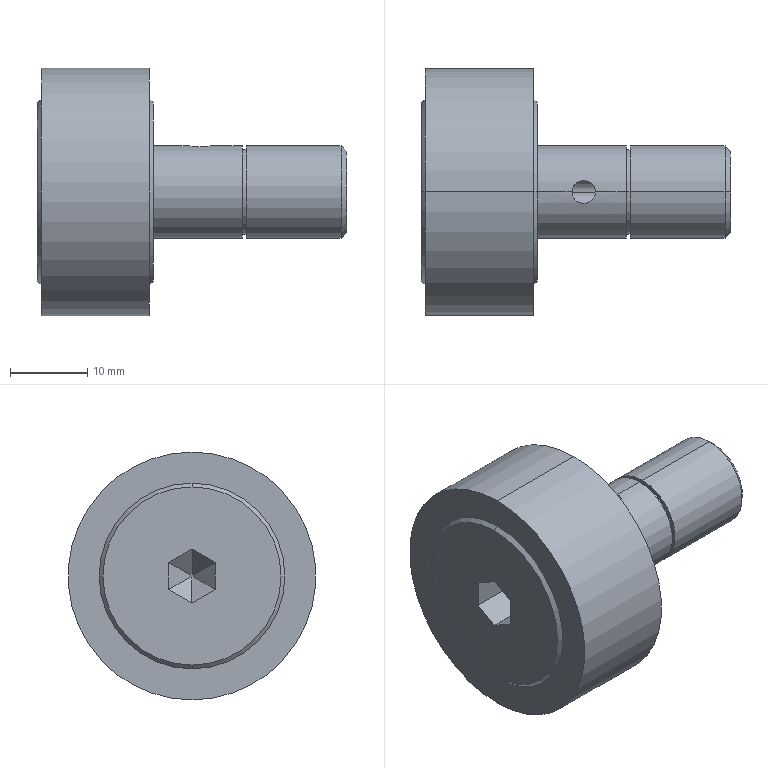Part | STEP file | BTL-01-32-0 | 1 solid | 43 faces | box 40 x 32 x 32 mm | volume 13951 mm3 | plane 21 | cylinder 14 | cone 8 | commonest cylinder face diameters 3 x4 12 x4 6 x2 11 x2 32 x2
STEP:
#1=CARTESIAN_POINT('',(7.,0.,16.));
#2=VERTEX_POINT('',#1);
#3=CARTESIAN_POINT('',(7.,0.,-16.));
#4=VERTEX_POINT('',#3);
#5=CARTESIAN_POINT('',(7.,0.,0.));
#6=DIRECTION('',(-1.,0.,0.));
#7=DIRECTION('',(0.,0.,1.));
#8=AXIS2_PLACEMENT_3D('',#5,#6,#7);
#9=CIRCLE('',#8,16.);
#10=EDGE_CURVE('',#2,#4,#9,.T.);
#11=ORIENTED_EDGE('',*,*,#10,.T.);
#12=CARTESIAN_POINT('',(-7.,0.,-16.));
#13=VERTEX_POINT('',#12);
#14=CARTESIAN_POINT('',(34.5,0.,-16.));
#15=DIRECTION('',(-1.,0.,0.));
#16=VECTOR('',#15,1000.);
#17=LINE('',#14,#16);
#18=EDGE_CURVE('',#4,#13,#17,.T.);
#19=ORIENTED_EDGE('',*,*,#18,.T.);
#20=CARTESIAN_POINT('',(-7.,0.,16.));
#21=VERTEX_POINT('',#20);
#22=CARTESIAN_POINT('',(-7.,0.,0.));
#23=DIRECTION('',(1.,0.,0.));
#24=DIRECTION('',(0.,0.,1.));
#25=AXIS2_PLACEMENT_3D('',#22,#23,#24);
#26=CIRCLE('',#25,16.);
#27=EDGE_CURVE('',#13,#21,#26,.T.);
#28=ORIENTED_EDGE('',*,*,#27,.T.);
#29=CARTESIAN_POINT('',(34.5,0.,16.));
#30=DIRECTION('',(-1.,0.,0.));
#31=VECTOR('',#30,1000.);
#32=LINE('',#29,#31);
#33=EDGE_CURVE('',#2,#21,#32,.T.);
#34=ORIENTED_EDGE('',*,*,#33,.F.);
#35=EDGE_LOOP('',(#11,#19,#28,#34));
#36=FACE_OUTER_BOUND('',#35,.T.);
#37=CARTESIAN_POINT('',(34.5,0.,0.));
#38=DIRECTION('',(-1.,0.,0.));
#39=DIRECTION('',(0.,0.,1.));
#40=AXIS2_PLACEMENT_3D('',#37,#38,#39);
#41=CYLINDRICAL_SURFACE('',#40,16.);
#42=ADVANCED_FACE('',(#36),#41,.T.);
#43=CARTESIAN_POINT('',(-7.5,0.,-11.5));
#44=VERTEX_POINT('',#43);
#45=CARTESIAN_POINT('',(-7.5,0.,11.5));
#46=VERTEX_POINT('',#45);
#47=CARTESIAN_POINT('',(-7.5,0.,0.));
#48=DIRECTION('',(1.,0.,0.));
#49=DIRECTION('',(0.,0.,-1.));
#50=AXIS2_PLACEMENT_3D('',#47,#48,#49);
#51=CIRCLE('',#50,11.5);
#52=EDGE_CURVE('',#44,#46,#51,.T.);
#53=ORIENTED_EDGE('',*,*,#52,.T.);
#54=CARTESIAN_POINT('',(-7.,0.,12.));
#55=VERTEX_POINT('',#54);
#56=CARTESIAN_POINT('',(-7.,0.,12.));
#57=DIRECTION('',(0.7071,0.,0.7071));
#58=VECTOR('',#57,1000.);
#59=LINE('',#56,#58);
#60=EDGE_CURVE('',#46,#55,#59,.T.);
#61=ORIENTED_EDGE('',*,*,#60,.T.);
#62=CARTESIAN_POINT('',(-7.,0.,-12.));
#63=VERTEX_POINT('',#62);
#64=CARTESIAN_POINT('',(-7.,0.,0.));
#65=DIRECTION('',(1.,0.,0.));
#66=DIRECTION('',(0.,0.,-1.));
#67=AXIS2_PLACEMENT_3D('',#64,#65,#66);
#68=CIRCLE('',#67,12.);
#69=EDGE_CURVE('',#63,#55,#68,.T.);
#70=ORIENTED_EDGE('',*,*,#69,.F.);
#71=CARTESIAN_POINT('',(-7.,0.,-12.));
#72=DIRECTION('',(0.7071,0.,-0.7071));
#73=VECTOR('',#72,1000.);
#74=LINE('',#71,#73);
#75=EDGE_CURVE('',#44,#63,#74,.T.);
#76=ORIENTED_EDGE('',*,*,#75,.F.);
#77=EDGE_LOOP('',(#53,#61,#70,#76));
#78=FACE_OUTER_BOUND('',#77,.T.);
#79=CARTESIAN_POINT('',(-7.,0.,0.));
#80=DIRECTION('',(1.,0.,0.));
#81=DIRECTION('',(0.,0.,-1.));
#82=AXIS2_PLACEMENT_3D('',#79,#80,#81);
#83=CONICAL_SURFACE('',#82,12.,0.7854);
#84=ADVANCED_FACE('',(#78),#83,.T.);
#85=CARTESIAN_POINT('',(7.5,0.,11.5));
#86=VERTEX_POINT('',#85);
#87=CARTESIAN_POINT('',(7.5,0.,-11.5));
#88=VERTEX_POINT('',#87);
#89=CARTESIAN_POINT('',(7.5,0.,0.));
#90=DIRECTION('',(-1.,0.,0.));
#91=DIRECTION('',(0.,0.,1.));
#92=AXIS2_PLACEMENT_3D('',#89,#90,#91);
#93=CIRCLE('',#92,11.5);
#94=EDGE_CURVE('',#86,#88,#93,.T.);
#95=ORIENTED_EDGE('',*,*,#94,.T.);
#96=CARTESIAN_POINT('',(7.,0.,-12.));
#97=VERTEX_POINT('',#96);
#98=CARTESIAN_POINT('',(7.,0.,-12.));
#99=DIRECTION('',(-0.7071,0.,-0.7071));
#100=VECTOR('',#99,1000.);
#101=LINE('',#98,#100);
#102=EDGE_CURVE('',#88,#97,#101,.T.);
#103=ORIENTED_EDGE('',*,*,#102,.T.);
#104=CARTESIAN_POINT('',(7.,0.,12.));
#105=VERTEX_POINT('',#104);
#106=CARTESIAN_POINT('',(7.,0.,0.));
#107=DIRECTION('',(1.,0.,0.));
#108=DIRECTION('',(0.,0.,1.));
#109=AXIS2_PLACEMENT_3D('',#106,#107,#108);
#110=CIRCLE('',#109,12.);
#111=EDGE_CURVE('',#97,#105,#110,.T.);
#112=ORIENTED_EDGE('',*,*,#111,.T.);
#113=CARTESIAN_POINT('',(7.,0.,12.));
#114=DIRECTION('',(-0.7071,0.,0.7071));
#115=VECTOR('',#114,1000.);
#116=LINE('',#113,#115);
#117=EDGE_CURVE('',#86,#105,#116,.T.);
#118=ORIENTED_EDGE('',*,*,#117,.F.);
#119=EDGE_LOOP('',(#95,#103,#112,#118));
#120=FACE_OUTER_BOUND('',#119,.T.);
#121=CARTESIAN_POINT('',(7.,0.,0.));
#122=DIRECTION('',(-1.,0.,0.));
#123=DIRECTION('',(0.,0.,1.));
#124=AXIS2_PLACEMENT_3D('',#121,#122,#123);
#125=CONICAL_SURFACE('',#124,12.,0.7854);
#126=ADVANCED_FACE('',(#120),#125,.T.);
#127=CARTESIAN_POINT('',(19.,0.,6.));
#128=VERTEX_POINT('',#127);
#129=CARTESIAN_POINT('',(19.,0.,-6.));
#130=VERTEX_POINT('',#129);
#131=CARTESIAN_POINT('',(19.,0.,0.));
#132=DIRECTION('',(-1.,0.,0.));
#133=DIRECTION('',(0.,0.,1.));
#134=AXIS2_PLACEMENT_3D('',#131,#132,#133);
#135=CIRCLE('',#134,6.);
#136=EDGE_CURVE('',#128,#130,#135,.T.);
#137=ORIENTED_EDGE('',*,*,#136,.T.);
#138=CARTESIAN_POINT('',(7.5,0.,-6.));
#139=VERTEX_POINT('',#138);
#140=CARTESIAN_POINT('',(34.5,0.,-6.));
#141=DIRECTION('',(-1.,0.,0.));
#142=VECTOR('',#141,1000.);
#143=LINE('',#140,#142);
#144=EDGE_CURVE('',#130,#139,#143,.T.);
#145=ORIENTED_EDGE('',*,*,#144,.T.);
#146=CARTESIAN_POINT('',(7.5,0.,6.));
#147=VERTEX_POINT('',#146);
#148=CARTESIAN_POINT('',(7.5,0.,0.));
#149=DIRECTION('',(1.,0.,0.));
#150=DIRECTION('',(0.,0.,1.));
#151=AXIS2_PLACEMENT_3D('',#148,#149,#150);
#152=CIRCLE('',#151,6.);
#153=EDGE_CURVE('',#139,#147,#152,.T.);
#154=ORIENTED_EDGE('',*,*,#153,.T.);
#155=CARTESIAN_POINT('',(12.,0.,6.));
#156=VERTEX_POINT('',#155);
#157=CARTESIAN_POINT('',(34.5,0.,6.));
#158=DIRECTION('',(-1.,0.,0.));
#159=VECTOR('',#158,1000.);
#160=LINE('',#157,#159);
#161=EDGE_CURVE('',#156,#147,#160,.T.);
#162=ORIENTED_EDGE('',*,*,#161,.F.);
#163=CARTESIAN_POINT('',(15.,0.,6.));
#164=VERTEX_POINT('',#163);
#165=CARTESIAN_POINT('',(12.,0.,6.));
#166=CARTESIAN_POINT('',(12.,0.09826,6.));
#167=CARTESIAN_POINT('',(12.01,0.1981,5.998));
#168=CARTESIAN_POINT('',(12.048,0.3907,5.988));
#169=CARTESIAN_POINT('',(12.077,0.4844,5.981));
#170=CARTESIAN_POINT('',(12.19,0.7575,5.955));
#171=CARTESIAN_POINT('',(12.301,0.9223,5.93));
#172=CARTESIAN_POINT('',(12.509,1.131,5.893));
#173=CARTESIAN_POINT('',(12.585,1.192,5.881));
#174=CARTESIAN_POINT('',(12.747,1.301,5.858));
#175=CARTESIAN_POINT('',(12.835,1.348,5.847));
#176=CARTESIAN_POINT('',(13.106,1.461,5.82));
#177=CARTESIAN_POINT('',(13.302,1.5,5.809));
#178=CARTESIAN_POINT('',(13.601,1.5,5.809));
#179=CARTESIAN_POINT('',(13.699,1.49,5.812));
#180=CARTESIAN_POINT('',(13.891,1.452,5.822));
#181=CARTESIAN_POINT('',(13.986,1.422,5.829));
#182=CARTESIAN_POINT('',(14.168,1.347,5.847));
#183=CARTESIAN_POINT('',(14.253,1.301,5.858));
#184=CARTESIAN_POINT('',(14.416,1.192,5.881));
#185=CARTESIAN_POINT('',(14.493,1.129,5.893));
#186=CARTESIAN_POINT('',(14.699,0.9219,5.93));
#187=CARTESIAN_POINT('',(14.811,0.7551,5.955));
#188=CARTESIAN_POINT('',(14.96,0.3944,5.99));
#189=CARTESIAN_POINT('',(15.,0.1965,6.));
#190=CARTESIAN_POINT('',(15.,0.,6.));
#191=B_SPLINE_CURVE_WITH_KNOTS('',3,(#165,#166,#167,#168,#169,#170,#171,#172,#173,#174,#175,#176,#177,#178,#179,#180,#181,#182,#183,#184,#185,#186,#187,#188,#189,#190),.UNSPECIFIED.,.F.,.F.,(4,2,2,2,2,2,2,2,2,2,2,2,4),(0.007062,0.007356,0.00765,0.008238,0.008533,0.008827,0.009415,0.009709,0.01,0.0103,0.01059,0.01118,0.01177),.UNSPECIFIED.);
#192=EDGE_CURVE('',#156,#164,#191,.T.);
#193=ORIENTED_EDGE('',*,*,#192,.T.);
#194=CARTESIAN_POINT('',(34.5,0.,6.));
#195=DIRECTION('',(-1.,0.,0.));
#196=VECTOR('',#195,1000.);
#197=LINE('',#194,#196);
#198=EDGE_CURVE('',#128,#164,#197,.T.);
#199=ORIENTED_EDGE('',*,*,#198,.F.);
#200=EDGE_LOOP('',(#137,#145,#154,#162,#193,#199));
#201=FACE_OUTER_BOUND('',#200,.T.);
#202=CARTESIAN_POINT('',(34.5,0.,0.));
#203=DIRECTION('',(-1.,0.,0.));
#204=DIRECTION('',(0.,0.,1.));
#205=AXIS2_PLACEMENT_3D('',#202,#203,#204);
#206=CYLINDRICAL_SURFACE('',#205,6.);
#207=ADVANCED_FACE('',(#201),#206,.T.);
#208=CARTESIAN_POINT('',(12.,0.,1.5));
#209=VERTEX_POINT('',#208);
#210=CARTESIAN_POINT('',(13.5,-1.5,0.));
#211=VERTEX_POINT('',#210);
#212=CARTESIAN_POINT('',(12.,0.,1.5));
#213=CARTESIAN_POINT('',(12.,-0.8787,1.5));
#214=CARTESIAN_POINT('',(12.621,-1.5,0.8787));
#215=CARTESIAN_POINT('',(13.5,-1.5,0.));
#216=(BOUNDED_CURVE()B_SPLINE_CURVE(3,(#212,#213,#214,#215),.UNSPECIFIED.,.F.,.F.)B_SPLINE_CURVE_WITH_KNOTS((4,4),(0.,1.571),.UNSPECIFIED.)CURVE()GEOMETRIC_REPRESENTATION_ITEM()RATIONAL_B_SPLINE_CURVE((1.,0.8047,0.8047,1.))REPRESENTATION_ITEM(''));
#217=EDGE_CURVE('',#209,#211,#216,.T.);
#218=ORIENTED_EDGE('',*,*,#217,.F.);
#219=CARTESIAN_POINT('',(12.,0.,-0.325));
#220=DIRECTION('',(0.,0.,1.));
#221=VECTOR('',#220,1000.);
#222=LINE('',#219,#221);
#223=EDGE_CURVE('',#209,#156,#222,.T.);
#224=ORIENTED_EDGE('',*,*,#223,.T.);
#225=CARTESIAN_POINT('',(15.,0.,6.));
#226=CARTESIAN_POINT('',(15.,-0.09825,6.));
#227=CARTESIAN_POINT('',(14.99,-0.1981,5.998));
#228=CARTESIAN_POINT('',(14.952,-0.3907,5.988));
#229=CARTESIAN_POINT('',(14.923,-0.4844,5.981));
#230=CARTESIAN_POINT('',(14.81,-0.7575,5.955));
#231=CARTESIAN_POINT('',(14.699,-0.9223,5.93));
#232=CARTESIAN_POINT('',(14.491,-1.131,5.893));
#233=CARTESIAN_POINT('',(14.415,-1.192,5.881));
#234=CARTESIAN_POINT('',(14.253,-1.301,5.858));
#235=CARTESIAN_POINT('',(14.165,-1.348,5.847));
#236=CARTESIAN_POINT('',(13.894,-1.461,5.82));
#237=CARTESIAN_POINT('',(13.698,-1.5,5.809));
#238=CARTESIAN_POINT('',(13.399,-1.5,5.809));
#239=CARTESIAN_POINT('',(13.301,-1.49,5.812));
#240=CARTESIAN_POINT('',(13.109,-1.452,5.822));
#241=CARTESIAN_POINT('',(13.014,-1.422,5.829));
#242=CARTESIAN_POINT('',(12.832,-1.347,5.847));
#243=CARTESIAN_POINT('',(12.747,-1.301,5.858));
#244=CARTESIAN_POINT('',(12.584,-1.192,5.881));
#245=CARTESIAN_POINT('',(12.507,-1.129,5.893));
#246=CARTESIAN_POINT('',(12.301,-0.9219,5.93));
#247=CARTESIAN_POINT('',(12.189,-0.7551,5.955));
#248=CARTESIAN_POINT('',(12.04,-0.3944,5.99));
#249=CARTESIAN_POINT('',(12.,-0.1965,6.));
#250=CARTESIAN_POINT('',(12.,0.,6.));
#251=B_SPLINE_CURVE_WITH_KNOTS('',3,(#225,#226,#227,#228,#229,#230,#231,#232,#233,#234,#235,#236,#237,#238,#239,#240,#241,#242,#243,#244,#245,#246,#247,#248,#249,#250),.UNSPECIFIED.,.F.,.F.,(4,2,2,2,2,2,2,2,2,2,2,2,4),(0.002355,0.002649,0.002943,0.003532,0.003826,0.00412,0.004708,0.005002,0.005297,0.005591,0.005885,0.006473,0.007062),.UNSPECIFIED.);
#252=EDGE_CURVE('',#164,#156,#251,.T.);
#253=ORIENTED_EDGE('',*,*,#252,.F.);
#254=CARTESIAN_POINT('',(15.,0.,1.5));
#255=VERTEX_POINT('',#254);
#256=CARTESIAN_POINT('',(15.,0.,-0.325));
#257=DIRECTION('',(0.,0.,1.));
#258=VECTOR('',#257,1000.);
#259=LINE('',#256,#258);
#260=EDGE_CURVE('',#255,#164,#259,.T.);
#261=ORIENTED_EDGE('',*,*,#260,.F.);
#262=CARTESIAN_POINT('',(13.5,-1.5,0.));
#263=CARTESIAN_POINT('',(14.379,-1.5,0.8787));
#264=CARTESIAN_POINT('',(15.,-0.8787,1.5));
#265=CARTESIAN_POINT('',(15.,0.,1.5));
#266=(BOUNDED_CURVE()B_SPLINE_CURVE(3,(#262,#263,#264,#265),.UNSPECIFIED.,.F.,.F.)B_SPLINE_CURVE_WITH_KNOTS((4,4),(1.571,3.142),.UNSPECIFIED.)CURVE()GEOMETRIC_REPRESENTATION_ITEM()RATIONAL_B_SPLINE_CURVE((1.,0.8047,0.8047,1.))REPRESENTATION_ITEM(''));
#267=EDGE_CURVE('',#211,#255,#266,.T.);
#268=ORIENTED_EDGE('',*,*,#267,.F.);
#269=EDGE_LOOP('',(#218,#224,#253,#261,#268));
#270=FACE_OUTER_BOUND('',#269,.T.);
#271=CARTESIAN_POINT('',(13.5,0.,-0.325));
#272=DIRECTION('',(0.,0.,1.));
#273=DIRECTION('',(1.,0.,0.));
#274=AXIS2_PLACEMENT_3D('',#271,#272,#273);
#275=CYLINDRICAL_SURFACE('',#274,1.5);
#276=ADVANCED_FACE('',(#270),#275,.F.);
#277=CARTESIAN_POINT('',(23.902,0.,-1.5));
#278=VERTEX_POINT('',#277);
#279=CARTESIAN_POINT('',(23.902,0.,1.5));
#280=VERTEX_POINT('',#279);
#281=CARTESIAN_POINT('',(23.902,0.,0.));
#282=DIRECTION('',(-1.,0.,0.));
#283=DIRECTION('',(0.,0.,1.));
#284=AXIS2_PLACEMENT_3D('',#281,#282,#283);
#285=CIRCLE('',#284,1.5);
#286=EDGE_CURVE('',#278,#280,#285,.T.);
#287=ORIENTED_EDGE('',*,*,#286,.F.);
#288=CARTESIAN_POINT('',(7.5,0.,-1.5));
#289=VERTEX_POINT('',#288);
#290=CARTESIAN_POINT('',(33.75,0.,-1.5));
#291=DIRECTION('',(-1.,0.,0.));
#292=VECTOR('',#291,1000.);
#293=LINE('',#290,#292);
#294=EDGE_CURVE('',#278,#289,#293,.T.);
#295=ORIENTED_EDGE('',*,*,#294,.T.);
#296=CARTESIAN_POINT('',(7.5,0.,1.5));
#297=VERTEX_POINT('',#296);
#298=CARTESIAN_POINT('',(7.5,0.,0.));
#299=DIRECTION('',(1.,0.,0.));
#300=DIRECTION('',(0.,0.,1.));
#301=AXIS2_PLACEMENT_3D('',#298,#299,#300);
#302=CIRCLE('',#301,1.5);
#303=EDGE_CURVE('',#297,#289,#302,.T.);
#304=ORIENTED_EDGE('',*,*,#303,.F.);
#305=CARTESIAN_POINT('',(33.75,0.,1.5));
#306=DIRECTION('',(-1.,0.,0.));
#307=VECTOR('',#306,1000.);
#308=LINE('',#305,#307);
#309=EDGE_CURVE('',#209,#297,#308,.T.);
#310=ORIENTED_EDGE('',*,*,#309,.F.);
#311=ORIENTED_EDGE('',*,*,#217,.T.);
#312=ORIENTED_EDGE('',*,*,#267,.T.);
#313=CARTESIAN_POINT('',(33.75,0.,1.5));
#314=DIRECTION('',(-1.,0.,0.));
#315=VECTOR('',#314,1000.);
#316=LINE('',#313,#315);
#317=EDGE_CURVE('',#280,#255,#316,.T.);
#318=ORIENTED_EDGE('',*,*,#317,.F.);
#319=EDGE_LOOP('',(#287,#295,#304,#310,#311,#312,#318));
#320=FACE_OUTER_BOUND('',#319,.T.);
#321=CARTESIAN_POINT('',(33.75,0.,0.));
#322=DIRECTION('',(-1.,0.,0.));
#323=DIRECTION('',(0.,0.,1.));
#324=AXIS2_PLACEMENT_3D('',#321,#322,#323);
#325=CYLINDRICAL_SURFACE('',#324,1.5);
#326=ADVANCED_FACE('',(#320),#325,.F.);
#327=CARTESIAN_POINT('',(19.5,0.,5.5));
#328=VERTEX_POINT('',#327);
#329=CARTESIAN_POINT('',(19.5,0.,-5.5));
#330=VERTEX_POINT('',#329);
#331=CARTESIAN_POINT('',(19.5,0.,0.));
#332=DIRECTION('',(-1.,0.,0.));
#333=DIRECTION('',(0.,0.,1.));
#334=AXIS2_PLACEMENT_3D('',#331,#332,#333);
#335=CIRCLE('',#334,5.5);
#336=EDGE_CURVE('',#328,#330,#335,.T.);
#337=ORIENTED_EDGE('',*,*,#336,.T.);
#338=CARTESIAN_POINT('',(19.,0.,-5.5));
#339=VERTEX_POINT('',#338);
#340=CARTESIAN_POINT('',(34.5,0.,-5.5));
#341=DIRECTION('',(-1.,0.,0.));
#342=VECTOR('',#341,1000.);
#343=LINE('',#340,#342);
#344=EDGE_CURVE('',#330,#339,#343,.T.);
#345=ORIENTED_EDGE('',*,*,#344,.T.);
#346=CARTESIAN_POINT('',(19.,0.,5.5));
#347=VERTEX_POINT('',#346);
#348=CARTESIAN_POINT('',(19.,0.,0.));
#349=DIRECTION('',(1.,0.,0.));
#350=DIRECTION('',(0.,0.,1.));
#351=AXIS2_PLACEMENT_3D('',#348,#349,#350);
#352=CIRCLE('',#351,5.5);
#353=EDGE_CURVE('',#339,#347,#352,.T.);
#354=ORIENTED_EDGE('',*,*,#353,.T.);
#355=CARTESIAN_POINT('',(34.5,0.,5.5));
#356=DIRECTION('',(-1.,0.,0.));
#357=VECTOR('',#356,1000.);
#358=LINE('',#355,#357);
#359=EDGE_CURVE('',#328,#347,#358,.T.);
#360=ORIENTED_EDGE('',*,*,#359,.F.);
#361=EDGE_LOOP('',(#337,#345,#354,#360));
#362=FACE_OUTER_BOUND('',#361,.T.);
#363=CARTESIAN_POINT('',(34.5,0.,0.));
#364=DIRECTION('',(-1.,0.,0.));
#365=DIRECTION('',(0.,0.,1.));
#366=AXIS2_PLACEMENT_3D('',#363,#364,#365);
#367=CYLINDRICAL_SURFACE('',#366,5.5);
#368=ADVANCED_FACE('',(#362),#367,.T.);
#369=ORIENTED_EDGE('',*,*,#286,.T.);
#370=CARTESIAN_POINT('',(26.5,0.,3.));
#371=VERTEX_POINT('',#370);
#372=CARTESIAN_POINT('',(26.5,0.,3.));
#373=DIRECTION('',(0.866,0.,0.5));
#374=VECTOR('',#373,1000.);
#375=LINE('',#372,#374);
#376=EDGE_CURVE('',#280,#371,#375,.T.);
#377=ORIENTED_EDGE('',*,*,#376,.T.);
#378=CARTESIAN_POINT('',(26.5,0.,-3.));
#379=VERTEX_POINT('',#378);
#380=CARTESIAN_POINT('',(26.5,0.,0.));
#381=DIRECTION('',(-1.,0.,0.));
#382=DIRECTION('',(0.,0.,1.));
#383=AXIS2_PLACEMENT_3D('',#380,#381,#382);
#384=CIRCLE('',#383,3.);
#385=EDGE_CURVE('',#379,#371,#384,.T.);
#386=ORIENTED_EDGE('',*,*,#385,.F.);
#387=CARTESIAN_POINT('',(26.5,0.,-3.));
#388=DIRECTION('',(0.866,0.,-0.5));
#389=VECTOR('',#388,1000.);
#390=LINE('',#387,#389);
#391=EDGE_CURVE('',#278,#379,#390,.T.);
#392=ORIENTED_EDGE('',*,*,#391,.F.);
#393=EDGE_LOOP('',(#369,#377,#386,#392));
#394=FACE_OUTER_BOUND('',#393,.T.);
#395=CARTESIAN_POINT('',(26.5,0.,0.));
#396=DIRECTION('',(1.,0.,0.));
#397=DIRECTION('',(0.,0.,-1.));
#398=AXIS2_PLACEMENT_3D('',#395,#396,#397);
#399=CONICAL_SURFACE('',#398,3.,0.5236);
#400=ADVANCED_FACE('',(#394),#399,.F.);
#401=CARTESIAN_POINT('',(32.5,0.,-3.));
#402=VERTEX_POINT('',#401);
#403=CARTESIAN_POINT('',(32.5,0.,3.));
#404=VERTEX_POINT('',#403);
#405=CARTESIAN_POINT('',(32.5,0.,0.));
#406=DIRECTION('',(-1.,0.,0.));
#407=DIRECTION('',(0.,0.,1.));
#408=AXIS2_PLACEMENT_3D('',#405,#406,#407);
#409=CIRCLE('',#408,3.);
#410=EDGE_CURVE('',#402,#404,#409,.T.);
#411=ORIENTED_EDGE('',*,*,#410,.F.);
#412=CARTESIAN_POINT('',(33.75,0.,-3.));
#413=DIRECTION('',(-1.,0.,0.));
#414=VECTOR('',#413,1000.);
#415=LINE('',#412,#414);
#416=EDGE_CURVE('',#402,#379,#415,.T.);
#417=ORIENTED_EDGE('',*,*,#416,.T.);
#418=ORIENTED_EDGE('',*,*,#385,.T.);
#419=CARTESIAN_POINT('',(33.75,0.,3.));
#420=DIRECTION('',(-1.,0.,0.));
#421=VECTOR('',#420,1000.);
#422=LINE('',#419,#421);
#423=EDGE_CURVE('',#404,#371,#422,.T.);
#424=ORIENTED_EDGE('',*,*,#423,.F.);
#425=EDGE_LOOP('',(#411,#417,#418,#424));
#426=FACE_OUTER_BOUND('',#425,.T.);
#427=CARTESIAN_POINT('',(33.75,0.,0.));
#428=DIRECTION('',(-1.,0.,0.));
#429=DIRECTION('',(0.,0.,1.));
#430=AXIS2_PLACEMENT_3D('',#427,#428,#429);
#431=CYLINDRICAL_SURFACE('',#430,3.);
#432=ADVANCED_FACE('',(#426),#431,.F.);
#433=CARTESIAN_POINT('',(31.75,0.,6.));
#434=VERTEX_POINT('',#433);
#435=CARTESIAN_POINT('',(31.75,0.,-6.));
#436=VERTEX_POINT('',#435);
#437=CARTESIAN_POINT('',(31.75,0.,0.));
#438=DIRECTION('',(-1.,0.,0.));
#439=DIRECTION('',(0.,0.,1.));
#440=AXIS2_PLACEMENT_3D('',#437,#438,#439);
#441=CIRCLE('',#440,6.);
#442=EDGE_CURVE('',#434,#436,#441,.T.);
#443=ORIENTED_EDGE('',*,*,#442,.T.);
#444=CARTESIAN_POINT('',(19.5,0.,-6.));
#445=VERTEX_POINT('',#444);
#446=CARTESIAN_POINT('',(34.5,0.,-6.));
#447=DIRECTION('',(-1.,0.,0.));
#448=VECTOR('',#447,1000.);
#449=LINE('',#446,#448);
#450=EDGE_CURVE('',#436,#445,#449,.T.);
#451=ORIENTED_EDGE('',*,*,#450,.T.);
#452=CARTESIAN_POINT('',(19.5,0.,6.));
#453=VERTEX_POINT('',#452);
#454=CARTESIAN_POINT('',(19.5,0.,0.));
#455=DIRECTION('',(-1.,0.,0.));
#456=DIRECTION('',(0.,0.,1.));
#457=AXIS2_PLACEMENT_3D('',#454,#455,#456);
#458=CIRCLE('',#457,6.);
#459=EDGE_CURVE('',#453,#445,#458,.T.);
#460=ORIENTED_EDGE('',*,*,#459,.F.);
#461=CARTESIAN_POINT('',(34.5,0.,6.));
#462=DIRECTION('',(-1.,0.,0.));
#463=VECTOR('',#462,1000.);
#464=LINE('',#461,#463);
#465=EDGE_CURVE('',#434,#453,#464,.T.);
#466=ORIENTED_EDGE('',*,*,#465,.F.);
#467=EDGE_LOOP('',(#443,#451,#460,#466));
#468=FACE_OUTER_BOUND('',#467,.T.);
#469=CARTESIAN_POINT('',(34.5,0.,0.));
#470=DIRECTION('',(-1.,0.,0.));
#471=DIRECTION('',(0.,0.,1.));
#472=AXIS2_PLACEMENT_3D('',#469,#470,#471);
#473=CYLINDRICAL_SURFACE('',#472,6.);
#474=ADVANCED_FACE('',(#468),#473,.T.);
#475=CARTESIAN_POINT('',(32.5,0.,5.25));
#476=VERTEX_POINT('',#475);
#477=CARTESIAN_POINT('',(32.5,0.,-5.25));
#478=VERTEX_POINT('',#477);
#479=CARTESIAN_POINT('',(32.5,0.,0.));
#480=DIRECTION('',(-1.,0.,0.));
#481=DIRECTION('',(0.,0.,1.));
#482=AXIS2_PLACEMENT_3D('',#479,#480,#481);
#483=CIRCLE('',#482,5.25);
#484=EDGE_CURVE('',#476,#478,#483,.T.);
#485=ORIENTED_EDGE('',*,*,#484,.T.);
#486=CARTESIAN_POINT('',(31.75,0.,-6.));
#487=DIRECTION('',(-0.7071,0.,-0.7071));
#488=VECTOR('',#487,1000.);
#489=LINE('',#486,#488);
#490=EDGE_CURVE('',#478,#436,#489,.T.);
#491=ORIENTED_EDGE('',*,*,#490,.T.);
#492=ORIENTED_EDGE('',*,*,#442,.F.);
#493=CARTESIAN_POINT('',(31.75,0.,6.));
#494=DIRECTION('',(-0.7071,0.,0.7071));
#495=VECTOR('',#494,1000.);
#496=LINE('',#493,#495);
#497=EDGE_CURVE('',#476,#434,#496,.T.);
#498=ORIENTED_EDGE('',*,*,#497,.F.);
#499=EDGE_LOOP('',(#485,#491,#492,#498));
#500=FACE_OUTER_BOUND('',#499,.T.);
#501=CARTESIAN_POINT('',(31.75,0.,0.));
#502=DIRECTION('',(-1.,0.,0.));
#503=DIRECTION('',(0.,0.,1.));
#504=AXIS2_PLACEMENT_3D('',#501,#502,#503);
#505=CONICAL_SURFACE('',#504,6.,0.7854);
#506=ADVANCED_FACE('',(#500),#505,.T.);
#507=ORIENTED_EDGE('',*,*,#18,.F.);
#508=CARTESIAN_POINT('',(7.,0.,0.));
#509=DIRECTION('',(-1.,0.,0.));
#510=DIRECTION('',(0.,0.,1.));
#511=AXIS2_PLACEMENT_3D('',#508,#509,#510);
#512=CIRCLE('',#511,16.);
#513=EDGE_CURVE('',#4,#2,#512,.T.);
#514=ORIENTED_EDGE('',*,*,#513,.T.);
#515=ORIENTED_EDGE('',*,*,#33,.T.);
#516=CARTESIAN_POINT('',(-7.,0.,0.));
#517=DIRECTION('',(1.,0.,0.));
#518=DIRECTION('',(0.,0.,1.));
#519=AXIS2_PLACEMENT_3D('',#516,#517,#518);
#520=CIRCLE('',#519,16.);
#521=EDGE_CURVE('',#21,#13,#520,.T.);
#522=ORIENTED_EDGE('',*,*,#521,.T.);
#523=EDGE_LOOP('',(#507,#514,#515,#522));
#524=FACE_OUTER_BOUND('',#523,.T.);
#525=CARTESIAN_POINT('',(34.5,0.,0.));
#526=DIRECTION('',(-1.,0.,0.));
#527=DIRECTION('',(0.,0.,1.));
#528=AXIS2_PLACEMENT_3D('',#525,#526,#527);
#529=CYLINDRICAL_SURFACE('',#528,16.);
#530=ADVANCED_FACE('',(#524),#529,.T.);
#531=ORIENTED_EDGE('',*,*,#69,.T.);
#532=CARTESIAN_POINT('',(-7.,0.,0.));
#533=DIRECTION('',(1.,0.,0.));
#534=DIRECTION('',(0.,0.,-1.));
#535=AXIS2_PLACEMENT_3D('',#532,#533,#534);
#536=CIRCLE('',#535,12.);
#537=EDGE_CURVE('',#55,#63,#536,.T.);
#538=ORIENTED_EDGE('',*,*,#537,.T.);
#539=EDGE_LOOP('',(#531,#538));
#540=FACE_BOUND('',#539,.T.);
#541=ORIENTED_EDGE('',*,*,#521,.F.);
#542=ORIENTED_EDGE('',*,*,#27,.F.);
#543=EDGE_LOOP('',(#541,#542));
#544=FACE_OUTER_BOUND('',#543,.T.);
#545=CARTESIAN_POINT('',(-7.,0.,0.));
#546=DIRECTION('',(-1.,0.,0.));
#547=DIRECTION('',(0.,0.,1.));
#548=AXIS2_PLACEMENT_3D('',#545,#546,#547);
#549=PLANE('',#548);
#550=ADVANCED_FACE('',(#540,#544),#549,.T.);
#551=CARTESIAN_POINT('',(7.,0.,0.));
#552=DIRECTION('',(1.,0.,0.));
#553=DIRECTION('',(0.,0.,1.));
#554=AXIS2_PLACEMENT_3D('',#551,#552,#553);
#555=CIRCLE('',#554,12.);
#556=EDGE_CURVE('',#105,#97,#555,.T.);
#557=ORIENTED_EDGE('',*,*,#556,.F.);
#558=ORIENTED_EDGE('',*,*,#111,.F.);
#559=EDGE_LOOP('',(#557,#558));
#560=FACE_BOUND('',#559,.T.);
#561=ORIENTED_EDGE('',*,*,#10,.F.);
#562=ORIENTED_EDGE('',*,*,#513,.F.);
#563=EDGE_LOOP('',(#561,#562));
#564=FACE_OUTER_BOUND('',#563,.T.);
#565=CARTESIAN_POINT('',(7.,0.,0.));
#566=DIRECTION('',(-1.,0.,0.));
#567=DIRECTION('',(0.,0.,1.));
#568=AXIS2_PLACEMENT_3D('',#565,#566,#567);
#569=PLANE('',#568);
#570=ADVANCED_FACE('',(#560,#564),#569,.F.);
#571=ORIENTED_EDGE('',*,*,#60,.F.);
#572=CARTESIAN_POINT('',(-7.5,0.,0.));
#573=DIRECTION('',(1.,0.,0.));
#574=DIRECTION('',(0.,0.,-1.));
#575=AXIS2_PLACEMENT_3D('',#572,#573,#574);
#576=CIRCLE('',#575,11.5);
#577=EDGE_CURVE('',#46,#44,#576,.T.);
#578=ORIENTED_EDGE('',*,*,#577,.T.);
#579=ORIENTED_EDGE('',*,*,#75,.T.);
#580=ORIENTED_EDGE('',*,*,#537,.F.);
#581=EDGE_LOOP('',(#571,#578,#579,#580));
#582=FACE_OUTER_BOUND('',#581,.T.);
#583=CARTESIAN_POINT('',(-7.,0.,0.));
#584=DIRECTION('',(1.,0.,0.));
#585=DIRECTION('',(0.,0.,-1.));
#586=AXIS2_PLACEMENT_3D('',#583,#584,#585);
#587=CONICAL_SURFACE('',#586,12.,0.7854);
#588=ADVANCED_FACE('',(#582),#587,.T.);
#589=ORIENTED_EDGE('',*,*,#102,.F.);
#590=CARTESIAN_POINT('',(7.5,0.,0.));
#591=DIRECTION('',(-1.,0.,0.));
#592=DIRECTION('',(0.,0.,1.));
#593=AXIS2_PLACEMENT_3D('',#590,#591,#592);
#594=CIRCLE('',#593,11.5);
#595=EDGE_CURVE('',#88,#86,#594,.T.);
#596=ORIENTED_EDGE('',*,*,#595,.T.);
#597=ORIENTED_EDGE('',*,*,#117,.T.);
#598=ORIENTED_EDGE('',*,*,#556,.T.);
#599=EDGE_LOOP('',(#589,#596,#597,#598));
#600=FACE_OUTER_BOUND('',#599,.T.);
#601=CARTESIAN_POINT('',(7.,0.,0.));
#602=DIRECTION('',(-1.,0.,0.));
#603=DIRECTION('',(0.,0.,1.));
#604=AXIS2_PLACEMENT_3D('',#601,#602,#603);
#605=CONICAL_SURFACE('',#604,12.,0.7854);
#606=ADVANCED_FACE('',(#600),#605,.T.);
#607=CARTESIAN_POINT('',(-7.5,-3.,1.732));
#608=VERTEX_POINT('',#607);
#609=CARTESIAN_POINT('',(-7.5,-3.,-1.732));
#610=VERTEX_POINT('',#609);
#611=CARTESIAN_POINT('',(-7.5,-3.,0.));
#612=DIRECTION('',(0.,0.,-1.));
#613=VECTOR('',#612,1000.);
#614=LINE('',#611,#613);
#615=EDGE_CURVE('',#608,#610,#614,.T.);
#616=ORIENTED_EDGE('',*,*,#615,.T.);
#617=CARTESIAN_POINT('',(-7.5,0.,-3.464));
#618=VERTEX_POINT('',#617);
#619=CARTESIAN_POINT('',(-7.5,-3.,-1.732));
#620=DIRECTION('',(0.,0.866,-0.5));
#621=VECTOR('',#620,1000.);
#622=LINE('',#619,#621);
#623=EDGE_CURVE('',#610,#618,#622,.T.);
#624=ORIENTED_EDGE('',*,*,#623,.T.);
#625=CARTESIAN_POINT('',(-7.5,3.,-1.732));
#626=VERTEX_POINT('',#625);
#627=CARTESIAN_POINT('',(-7.5,0.,-3.464));
#628=DIRECTION('',(0.,0.866,0.5));
#629=VECTOR('',#628,1000.);
#630=LINE('',#627,#629);
#631=EDGE_CURVE('',#618,#626,#630,.T.);
#632=ORIENTED_EDGE('',*,*,#631,.T.);
#633=CARTESIAN_POINT('',(-7.5,3.,1.732));
#634=VERTEX_POINT('',#633);
#635=CARTESIAN_POINT('',(-7.5,3.,0.));
#636=DIRECTION('',(0.,0.,1.));
#637=VECTOR('',#636,1000.);
#638=LINE('',#635,#637);
#639=EDGE_CURVE('',#626,#634,#638,.T.);
#640=ORIENTED_EDGE('',*,*,#639,.T.);
#641=CARTESIAN_POINT('',(-7.5,0.,3.464));
#642=VERTEX_POINT('',#641);
#643=CARTESIAN_POINT('',(-7.5,3.,1.732));
#644=DIRECTION('',(0.,-0.866,0.5));
#645=VECTOR('',#644,1000.);
#646=LINE('',#643,#645);
#647=EDGE_CURVE('',#634,#642,#646,.T.);
#648=ORIENTED_EDGE('',*,*,#647,.T.);
#649=CARTESIAN_POINT('',(-7.5,0.,3.464));
#650=DIRECTION('',(0.,-0.866,-0.5));
#651=VECTOR('',#650,1000.);
#652=LINE('',#649,#651);
#653=EDGE_CURVE('',#642,#608,#652,.T.);
#654=ORIENTED_EDGE('',*,*,#653,.T.);
#655=EDGE_LOOP('',(#616,#624,#632,#640,#648,#654));
#656=FACE_BOUND('',#655,.T.);
#657=ORIENTED_EDGE('',*,*,#52,.F.);
#658=ORIENTED_EDGE('',*,*,#577,.F.);
#659=EDGE_LOOP('',(#657,#658));
#660=FACE_OUTER_BOUND('',#659,.T.);
#661=CARTESIAN_POINT('',(-7.5,0.,0.));
#662=DIRECTION('',(-1.,0.,0.));
#663=DIRECTION('',(0.,0.,1.));
#664=AXIS2_PLACEMENT_3D('',#661,#662,#663);
#665=PLANE('',#664);
#666=ADVANCED_FACE('',(#656,#660),#665,.T.);
#667=CARTESIAN_POINT('',(7.5,0.,0.));
#668=DIRECTION('',(1.,0.,0.));
#669=DIRECTION('',(0.,0.,1.));
#670=AXIS2_PLACEMENT_3D('',#667,#668,#669);
#671=CIRCLE('',#670,6.);
#672=EDGE_CURVE('',#147,#139,#671,.T.);
#673=ORIENTED_EDGE('',*,*,#672,.F.);
#674=ORIENTED_EDGE('',*,*,#153,.F.);
#675=EDGE_LOOP('',(#673,#674));
#676=FACE_BOUND('',#675,.T.);
#677=ORIENTED_EDGE('',*,*,#94,.F.);
#678=ORIENTED_EDGE('',*,*,#595,.F.);
#679=EDGE_LOOP('',(#677,#678));
#680=FACE_OUTER_BOUND('',#679,.T.);
#681=CARTESIAN_POINT('',(7.5,0.,0.));
#682=DIRECTION('',(-1.,0.,0.));
#683=DIRECTION('',(0.,0.,1.));
#684=AXIS2_PLACEMENT_3D('',#681,#682,#683);
#685=PLANE('',#684);
#686=ADVANCED_FACE('',(#676,#680),#685,.F.);
#687=ORIENTED_EDGE('',*,*,#623,.F.);
#688=CARTESIAN_POINT('',(-2.5,-3.,-1.732));
#689=VERTEX_POINT('',#688);
#690=CARTESIAN_POINT('',(-7.5,-3.,-1.732));
#691=DIRECTION('',(-1.,0.,0.));
#692=VECTOR('',#691,1000.);
#693=LINE('',#690,#692);
#694=EDGE_CURVE('',#689,#610,#693,.T.);
#695=ORIENTED_EDGE('',*,*,#694,.F.);
#696=CARTESIAN_POINT('',(-2.5,0.,-3.464));
#697=VERTEX_POINT('',#696);
#698=CARTESIAN_POINT('',(-2.5,0.,-3.464));
#699=DIRECTION('',(0.,-0.866,0.5));
#700=VECTOR('',#699,1000.);
#701=LINE('',#698,#700);
#702=EDGE_CURVE('',#697,#689,#701,.T.);
#703=ORIENTED_EDGE('',*,*,#702,.F.);
#704=CARTESIAN_POINT('',(-7.5,0.,-3.464));
#705=DIRECTION('',(1.,0.,0.));
#706=VECTOR('',#705,1000.);
#707=LINE('',#704,#706);
#708=EDGE_CURVE('',#618,#697,#707,.T.);
#709=ORIENTED_EDGE('',*,*,#708,.F.);
#710=EDGE_LOOP('',(#687,#695,#703,#709));
#711=FACE_OUTER_BOUND('',#710,.T.);
#712=CARTESIAN_POINT('',(-7.5,0.,-3.464));
#713=DIRECTION('',(0.,-0.5,-0.866));
#714=DIRECTION('',(0.,0.866,-0.5));
#715=AXIS2_PLACEMENT_3D('',#712,#713,#714);
#716=PLANE('',#715);
#717=ADVANCED_FACE('',(#711),#716,.F.);
#718=ORIENTED_EDGE('',*,*,#615,.F.);
#719=CARTESIAN_POINT('',(-2.5,-3.,1.732));
#720=VERTEX_POINT('',#719);
#721=CARTESIAN_POINT('',(-7.5,-3.,1.732));
#722=DIRECTION('',(-1.,0.,0.));
#723=VECTOR('',#722,1000.);
#724=LINE('',#721,#723);
#725=EDGE_CURVE('',#720,#608,#724,.T.);
#726=ORIENTED_EDGE('',*,*,#725,.F.);
#727=CARTESIAN_POINT('',(-2.5,-3.,-1.732));
#728=DIRECTION('',(0.,0.,1.));
#729=VECTOR('',#728,1000.);
#730=LINE('',#727,#729);
#731=EDGE_CURVE('',#689,#720,#730,.T.);
#732=ORIENTED_EDGE('',*,*,#731,.F.);
#733=ORIENTED_EDGE('',*,*,#694,.T.);
#734=EDGE_LOOP('',(#718,#726,#732,#733));
#735=FACE_OUTER_BOUND('',#734,.T.);
#736=CARTESIAN_POINT('',(-7.5,-3.,-1.732));
#737=DIRECTION('',(0.,-1.,0.));
#738=DIRECTION('',(0.,0.,-1.));
#739=AXIS2_PLACEMENT_3D('',#736,#737,#738);
#740=PLANE('',#739);
#741=ADVANCED_FACE('',(#735),#740,.F.);
#742=ORIENTED_EDGE('',*,*,#653,.F.);
#743=CARTESIAN_POINT('',(-2.5,0.,3.464));
#744=VERTEX_POINT('',#743);
#745=CARTESIAN_POINT('',(-7.5,0.,3.464));
#746=DIRECTION('',(-1.,0.,0.));
#747=VECTOR('',#746,1000.);
#748=LINE('',#745,#747);
#749=EDGE_CURVE('',#744,#642,#748,.T.);
#750=ORIENTED_EDGE('',*,*,#749,.F.);
#751=CARTESIAN_POINT('',(-2.5,-3.,1.732));
#752=DIRECTION('',(0.,0.866,0.5));
#753=VECTOR('',#752,1000.);
#754=LINE('',#751,#753);
#755=EDGE_CURVE('',#720,#744,#754,.T.);
#756=ORIENTED_EDGE('',*,*,#755,.F.);
#757=ORIENTED_EDGE('',*,*,#725,.T.);
#758=EDGE_LOOP('',(#742,#750,#756,#757));
#759=FACE_OUTER_BOUND('',#758,.T.);
#760=CARTESIAN_POINT('',(-7.5,-3.,1.732));
#761=DIRECTION('',(0.,-0.5,0.866));
#762=DIRECTION('',(0.,-0.866,-0.5));
#763=AXIS2_PLACEMENT_3D('',#760,#761,#762);
#764=PLANE('',#763);
#765=ADVANCED_FACE('',(#759),#764,.F.);
#766=ORIENTED_EDGE('',*,*,#647,.F.);
#767=CARTESIAN_POINT('',(-2.5,3.,1.732));
#768=VERTEX_POINT('',#767);
#769=CARTESIAN_POINT('',(-7.5,3.,1.732));
#770=DIRECTION('',(-1.,0.,0.));
#771=VECTOR('',#770,1000.);
#772=LINE('',#769,#771);
#773=EDGE_CURVE('',#768,#634,#772,.T.);
#774=ORIENTED_EDGE('',*,*,#773,.F.);
#775=CARTESIAN_POINT('',(-2.5,0.,3.464));
#776=DIRECTION('',(0.,0.866,-0.5));
#777=VECTOR('',#776,1000.);
#778=LINE('',#775,#777);
#779=EDGE_CURVE('',#744,#768,#778,.T.);
#780=ORIENTED_EDGE('',*,*,#779,.F.);
#781=ORIENTED_EDGE('',*,*,#749,.T.);
#782=EDGE_LOOP('',(#766,#774,#780,#781));
#783=FACE_OUTER_BOUND('',#782,.T.);
#784=CARTESIAN_POINT('',(-7.5,0.,3.464));
#785=DIRECTION('',(0.,0.5,0.866));
#786=DIRECTION('',(0.,-0.866,0.5));
#787=AXIS2_PLACEMENT_3D('',#784,#785,#786);
#788=PLANE('',#787);
#789=ADVANCED_FACE('',(#783),#788,.F.);
#790=ORIENTED_EDGE('',*,*,#639,.F.);
#791=CARTESIAN_POINT('',(-2.5,3.,-1.732));
#792=VERTEX_POINT('',#791);
#793=CARTESIAN_POINT('',(-7.5,3.,-1.732));
#794=DIRECTION('',(-1.,0.,0.));
#795=VECTOR('',#794,1000.);
#796=LINE('',#793,#795);
#797=EDGE_CURVE('',#792,#626,#796,.T.);
#798=ORIENTED_EDGE('',*,*,#797,.F.);
#799=CARTESIAN_POINT('',(-2.5,3.,1.732));
#800=DIRECTION('',(0.,0.,-1.));
#801=VECTOR('',#800,1000.);
#802=LINE('',#799,#801);
#803=EDGE_CURVE('',#768,#792,#802,.T.);
#804=ORIENTED_EDGE('',*,*,#803,.F.);
#805=ORIENTED_EDGE('',*,*,#773,.T.);
#806=EDGE_LOOP('',(#790,#798,#804,#805));
#807=FACE_OUTER_BOUND('',#806,.T.);
#808=CARTESIAN_POINT('',(-7.5,3.,1.732));
#809=DIRECTION('',(0.,1.,0.));
#810=DIRECTION('',(0.,0.,1.));
#811=AXIS2_PLACEMENT_3D('',#808,#809,#810);
#812=PLANE('',#811);
#813=ADVANCED_FACE('',(#807),#812,.F.);
#814=ORIENTED_EDGE('',*,*,#631,.F.);
#815=ORIENTED_EDGE('',*,*,#708,.T.);
#816=CARTESIAN_POINT('',(-2.5,3.,-1.732));
#817=DIRECTION('',(0.,-0.866,-0.5));
#818=VECTOR('',#817,1000.);
#819=LINE('',#816,#818);
#820=EDGE_CURVE('',#792,#697,#819,.T.);
#821=ORIENTED_EDGE('',*,*,#820,.F.);
#822=ORIENTED_EDGE('',*,*,#797,.T.);
#823=EDGE_LOOP('',(#814,#815,#821,#822));
#824=FACE_OUTER_BOUND('',#823,.T.);
#825=CARTESIAN_POINT('',(-7.5,3.,-1.732));
#826=DIRECTION('',(0.,0.5,-0.866));
#827=DIRECTION('',(0.,0.866,0.5));
#828=AXIS2_PLACEMENT_3D('',#825,#826,#827);
#829=PLANE('',#828);
#830=ADVANCED_FACE('',(#824),#829,.F.);
#831=ORIENTED_EDGE('',*,*,#144,.F.);
#832=CARTESIAN_POINT('',(19.,0.,0.));
#833=DIRECTION('',(-1.,0.,0.));
#834=DIRECTION('',(0.,0.,1.));
#835=AXIS2_PLACEMENT_3D('',#832,#833,#834);
#836=CIRCLE('',#835,6.);
#837=EDGE_CURVE('',#130,#128,#836,.T.);
#838=ORIENTED_EDGE('',*,*,#837,.T.);
#839=ORIENTED_EDGE('',*,*,#198,.T.);
#840=ORIENTED_EDGE('',*,*,#252,.T.);
#841=ORIENTED_EDGE('',*,*,#161,.T.);
#842=ORIENTED_EDGE('',*,*,#672,.T.);
#843=EDGE_LOOP('',(#831,#838,#839,#840,#841,#842));
#844=FACE_OUTER_BOUND('',#843,.T.);
#845=CARTESIAN_POINT('',(34.5,0.,0.));
#846=DIRECTION('',(-1.,0.,0.));
#847=DIRECTION('',(0.,0.,1.));
#848=AXIS2_PLACEMENT_3D('',#845,#846,#847);
#849=CYLINDRICAL_SURFACE('',#848,6.);
#850=ADVANCED_FACE('',(#844),#849,.T.);
#851=CARTESIAN_POINT('',(0.5,0.,-0.25));
#852=VERTEX_POINT('',#851);
#853=CARTESIAN_POINT('',(0.5,-0.2165,-0.125));
#854=VERTEX_POINT('',#853);
#855=CARTESIAN_POINT('',(0.5,0.,-0.25));
#856=DIRECTION('',(0.,-0.866,0.5));
#857=VECTOR('',#856,1000.);
#858=LINE('',#855,#857);
#859=EDGE_CURVE('',#852,#854,#858,.T.);
#860=ORIENTED_EDGE('',*,*,#859,.F.);
#861=CARTESIAN_POINT('',(-0.7684,0.,-1.609));
#862=DIRECTION('',(0.6823,0.,0.731));
#863=VECTOR('',#862,1000.);
#864=LINE('',#861,#863);
#865=EDGE_CURVE('',#697,#852,#864,.T.);
#866=ORIENTED_EDGE('',*,*,#865,.F.);
#867=ORIENTED_EDGE('',*,*,#702,.T.);
#868=CARTESIAN_POINT('',(0.5,-0.2165,-0.125));
#869=DIRECTION('',(-0.6823,-0.6331,-0.3655));
#870=VECTOR('',#869,1000.);
#871=LINE('',#868,#870);
#872=EDGE_CURVE('',#854,#689,#871,.T.);
#873=ORIENTED_EDGE('',*,*,#872,.F.);
#874=EDGE_LOOP('',(#860,#866,#867,#873));
#875=FACE_OUTER_BOUND('',#874,.T.);
#876=CARTESIAN_POINT('',(-1.,-0.8041,-1.393));
#877=DIRECTION('',(0.6802,-0.3665,-0.6349));
#878=DIRECTION('',(-0.6823,0.,-0.731));
#879=AXIS2_PLACEMENT_3D('',#876,#877,#878);
#880=PLANE('',#879);
#881=ADVANCED_FACE('',(#875),#880,.F.);
#882=CARTESIAN_POINT('',(0.5,-0.2165,0.125));
#883=VERTEX_POINT('',#882);
#884=CARTESIAN_POINT('',(0.5,-0.2165,0.));
#885=DIRECTION('',(0.,0.,1.));
#886=VECTOR('',#885,1000.);
#887=LINE('',#884,#886);
#888=EDGE_CURVE('',#854,#883,#887,.T.);
#889=ORIENTED_EDGE('',*,*,#888,.F.);
#890=ORIENTED_EDGE('',*,*,#872,.T.);
#891=ORIENTED_EDGE('',*,*,#731,.T.);
#892=CARTESIAN_POINT('',(0.5,-0.2165,0.125));
#893=DIRECTION('',(-0.6823,-0.6331,0.3655));
#894=VECTOR('',#893,1000.);
#895=LINE('',#892,#894);
#896=EDGE_CURVE('',#883,#720,#895,.T.);
#897=ORIENTED_EDGE('',*,*,#896,.F.);
#898=EDGE_LOOP('',(#889,#890,#891,#897));
#899=FACE_OUTER_BOUND('',#898,.T.);
#900=CARTESIAN_POINT('',(-1.,-1.608,0.));
#901=DIRECTION('',(0.6802,-0.7331,0.));
#902=DIRECTION('',(0.7331,0.6802,0.));
#903=AXIS2_PLACEMENT_3D('',#900,#901,#902);
#904=PLANE('',#903);
#905=ADVANCED_FACE('',(#899),#904,.F.);
#906=CARTESIAN_POINT('',(0.5,0.,0.25));
#907=VERTEX_POINT('',#906);
#908=CARTESIAN_POINT('',(0.5,-0.2165,0.125));
#909=DIRECTION('',(0.,0.866,0.5));
#910=VECTOR('',#909,1000.);
#911=LINE('',#908,#910);
#912=EDGE_CURVE('',#883,#907,#911,.T.);
#913=ORIENTED_EDGE('',*,*,#912,.F.);
#914=ORIENTED_EDGE('',*,*,#896,.T.);
#915=ORIENTED_EDGE('',*,*,#755,.T.);
#916=CARTESIAN_POINT('',(-0.7684,0.,1.609));
#917=DIRECTION('',(-0.6823,0.,0.731));
#918=VECTOR('',#917,1000.);
#919=LINE('',#916,#918);
#920=EDGE_CURVE('',#907,#744,#919,.T.);
#921=ORIENTED_EDGE('',*,*,#920,.F.);
#922=EDGE_LOOP('',(#913,#914,#915,#921));
#923=FACE_OUTER_BOUND('',#922,.T.);
#924=CARTESIAN_POINT('',(-1.,-0.8041,1.393));
#925=DIRECTION('',(0.6802,-0.3665,0.6349));
#926=DIRECTION('',(0.6823,0.,-0.731));
#927=AXIS2_PLACEMENT_3D('',#924,#925,#926);
#928=PLANE('',#927);
#929=ADVANCED_FACE('',(#923),#928,.F.);
#930=CARTESIAN_POINT('',(0.5,0.2165,0.125));
#931=VERTEX_POINT('',#930);
#932=CARTESIAN_POINT('',(0.5,0.,0.25));
#933=DIRECTION('',(0.,0.866,-0.5));
#934=VECTOR('',#933,1000.);
#935=LINE('',#932,#934);
#936=EDGE_CURVE('',#907,#931,#935,.T.);
#937=ORIENTED_EDGE('',*,*,#936,.F.);
#938=ORIENTED_EDGE('',*,*,#920,.T.);
#939=ORIENTED_EDGE('',*,*,#779,.T.);
#940=CARTESIAN_POINT('',(0.5,0.2165,0.125));
#941=DIRECTION('',(-0.6823,0.6331,0.3655));
#942=VECTOR('',#941,1000.);
#943=LINE('',#940,#942);
#944=EDGE_CURVE('',#931,#768,#943,.T.);
#945=ORIENTED_EDGE('',*,*,#944,.F.);
#946=EDGE_LOOP('',(#937,#938,#939,#945));
#947=FACE_OUTER_BOUND('',#946,.T.);
#948=CARTESIAN_POINT('',(-1.,0.8041,1.393));
#949=DIRECTION('',(0.6802,0.3665,0.6349));
#950=DIRECTION('',(0.6823,0.,-0.731));
#951=AXIS2_PLACEMENT_3D('',#948,#949,#950);
#952=PLANE('',#951);
#953=ADVANCED_FACE('',(#947),#952,.F.);
#954=CARTESIAN_POINT('',(0.5,0.2165,-0.125));
#955=VERTEX_POINT('',#954);
#956=CARTESIAN_POINT('',(0.5,0.2165,0.));
#957=DIRECTION('',(0.,0.,-1.));
#958=VECTOR('',#957,1000.);
#959=LINE('',#956,#958);
#960=EDGE_CURVE('',#931,#955,#959,.T.);
#961=ORIENTED_EDGE('',*,*,#960,.F.);
#962=ORIENTED_EDGE('',*,*,#944,.T.);
#963=ORIENTED_EDGE('',*,*,#803,.T.);
#964=CARTESIAN_POINT('',(0.5,0.2165,-0.125));
#965=DIRECTION('',(-0.6823,0.6331,-0.3655));
#966=VECTOR('',#965,1000.);
#967=LINE('',#964,#966);
#968=EDGE_CURVE('',#955,#792,#967,.T.);
#969=ORIENTED_EDGE('',*,*,#968,.F.);
#970=EDGE_LOOP('',(#961,#962,#963,#969));
#971=FACE_OUTER_BOUND('',#970,.T.);
#972=CARTESIAN_POINT('',(-1.,1.608,0.));
#973=DIRECTION('',(0.6802,0.7331,0.));
#974=DIRECTION('',(-0.7331,0.6802,0.));
#975=AXIS2_PLACEMENT_3D('',#972,#973,#974);
#976=PLANE('',#975);
#977=ADVANCED_FACE('',(#971),#976,.F.);
#978=CARTESIAN_POINT('',(0.5,0.2165,-0.125));
#979=DIRECTION('',(0.,-0.866,-0.5));
#980=VECTOR('',#979,1000.);
#981=LINE('',#978,#980);
#982=EDGE_CURVE('',#955,#852,#981,.T.);
#983=ORIENTED_EDGE('',*,*,#982,.F.);
#984=ORIENTED_EDGE('',*,*,#968,.T.);
#985=ORIENTED_EDGE('',*,*,#820,.T.);
#986=ORIENTED_EDGE('',*,*,#865,.T.);
#987=EDGE_LOOP('',(#983,#984,#985,#986));
#988=FACE_OUTER_BOUND('',#987,.T.);
#989=CARTESIAN_POINT('',(-1.,0.8041,-1.393));
#990=DIRECTION('',(0.6802,0.3665,-0.6349));
#991=DIRECTION('',(-0.6823,0.,-0.731));
#992=AXIS2_PLACEMENT_3D('',#989,#990,#991);
#993=PLANE('',#992);
#994=ADVANCED_FACE('',(#988),#993,.F.);
#995=ORIENTED_EDGE('',*,*,#223,.F.);
#996=CARTESIAN_POINT('',(13.5,1.5,0.));
#997=VERTEX_POINT('',#996);
#998=CARTESIAN_POINT('',(13.5,1.5,0.));
#999=CARTESIAN_POINT('',(12.621,1.5,0.8787));
#1000=CARTESIAN_POINT('',(12.,0.8787,1.5));
#1001=CARTESIAN_POINT('',(12.,0.,1.5));
#1002=(BOUNDED_CURVE()B_SPLINE_CURVE(3,(#998,#999,#1000,#1001),.UNSPECIFIED.,.F.,.T.)B_SPLINE_CURVE_WITH_KNOTS((4,4),(4.712,6.283),.UNSPECIFIED.)CURVE()GEOMETRIC_REPRESENTATION_ITEM()RATIONAL_B_SPLINE_CURVE((1.,0.8047,0.8047,1.))REPRESENTATION_ITEM(''));
#1003=EDGE_CURVE('',#997,#209,#1002,.T.);
#1004=ORIENTED_EDGE('',*,*,#1003,.F.);
#1005=CARTESIAN_POINT('',(15.,0.,1.5));
#1006=CARTESIAN_POINT('',(15.,0.8787,1.5));
#1007=CARTESIAN_POINT('',(14.379,1.5,0.8787));
#1008=CARTESIAN_POINT('',(13.5,1.5,0.));
#1009=(BOUNDED_CURVE()B_SPLINE_CURVE(3,(#1005,#1006,#1007,#1008),.UNSPECIFIED.,.F.,.T.)B_SPLINE_CURVE_WITH_KNOTS((4,4),(3.142,4.712),.UNSPECIFIED.)CURVE()GEOMETRIC_REPRESENTATION_ITEM()RATIONAL_B_SPLINE_CURVE((1.,0.8047,0.8047,1.))REPRESENTATION_ITEM(''));
#1010=EDGE_CURVE('',#255,#997,#1009,.T.);
#1011=ORIENTED_EDGE('',*,*,#1010,.F.);
#1012=ORIENTED_EDGE('',*,*,#260,.T.);
#1013=ORIENTED_EDGE('',*,*,#192,.F.);
#1014=EDGE_LOOP('',(#995,#1004,#1011,#1012,#1013));
#1015=FACE_OUTER_BOUND('',#1014,.T.);
#1016=CARTESIAN_POINT('',(13.5,0.,-0.325));
#1017=DIRECTION('',(0.,0.,1.));
#1018=DIRECTION('',(1.,0.,0.));
#1019=AXIS2_PLACEMENT_3D('',#1016,#1017,#1018);
#1020=CYLINDRICAL_SURFACE('',#1019,1.5);
#1021=ADVANCED_FACE('',(#1015),#1020,.F.);
#1022=CARTESIAN_POINT('',(19.,0.,0.));
#1023=DIRECTION('',(1.,0.,0.));
#1024=DIRECTION('',(0.,0.,1.));
#1025=AXIS2_PLACEMENT_3D('',#1022,#1023,#1024);
#1026=CIRCLE('',#1025,5.5);
#1027=EDGE_CURVE('',#347,#339,#1026,.T.);
#1028=ORIENTED_EDGE('',*,*,#1027,.F.);
#1029=ORIENTED_EDGE('',*,*,#353,.F.);
#1030=EDGE_LOOP('',(#1028,#1029));
#1031=FACE_BOUND('',#1030,.T.);
#1032=ORIENTED_EDGE('',*,*,#136,.F.);
#1033=ORIENTED_EDGE('',*,*,#837,.F.);
#1034=EDGE_LOOP('',(#1032,#1033));
#1035=FACE_OUTER_BOUND('',#1034,.T.);
#1036=CARTESIAN_POINT('',(19.,0.,0.));
#1037=DIRECTION('',(-1.,0.,0.));
#1038=DIRECTION('',(0.,0.,1.));
#1039=AXIS2_PLACEMENT_3D('',#1036,#1037,#1038);
#1040=PLANE('',#1039);
#1041=ADVANCED_FACE('',(#1031,#1035),#1040,.F.);
#1042=ORIENTED_EDGE('',*,*,#982,.T.);
#1043=ORIENTED_EDGE('',*,*,#859,.T.);
#1044=ORIENTED_EDGE('',*,*,#888,.T.);
#1045=ORIENTED_EDGE('',*,*,#912,.T.);
#1046=ORIENTED_EDGE('',*,*,#936,.T.);
#1047=ORIENTED_EDGE('',*,*,#960,.T.);
#1048=EDGE_LOOP('',(#1042,#1043,#1044,#1045,#1046,#1047));
#1049=FACE_OUTER_BOUND('',#1048,.T.);
#1050=CARTESIAN_POINT('',(0.5,0.,0.));
#1051=DIRECTION('',(-1.,0.,0.));
#1052=DIRECTION('',(0.,0.,1.));
#1053=AXIS2_PLACEMENT_3D('',#1050,#1051,#1052);
#1054=PLANE('',#1053);
#1055=ADVANCED_FACE('',(#1049),#1054,.T.);
#1056=ORIENTED_EDGE('',*,*,#294,.F.);
#1057=CARTESIAN_POINT('',(23.902,0.,0.));
#1058=DIRECTION('',(-1.,0.,0.));
#1059=DIRECTION('',(0.,0.,1.));
#1060=AXIS2_PLACEMENT_3D('',#1057,#1058,#1059);
#1061=CIRCLE('',#1060,1.5);
#1062=EDGE_CURVE('',#280,#278,#1061,.T.);
#1063=ORIENTED_EDGE('',*,*,#1062,.F.);
#1064=ORIENTED_EDGE('',*,*,#317,.T.);
#1065=ORIENTED_EDGE('',*,*,#1010,.T.);
#1066=ORIENTED_EDGE('',*,*,#1003,.T.);
#1067=ORIENTED_EDGE('',*,*,#309,.T.);
#1068=CARTESIAN_POINT('',(7.5,0.,0.));
#1069=DIRECTION('',(1.,0.,0.));
#1070=DIRECTION('',(0.,0.,1.));
#1071=AXIS2_PLACEMENT_3D('',#1068,#1069,#1070);
#1072=CIRCLE('',#1071,1.5);
#1073=EDGE_CURVE('',#289,#297,#1072,.T.);
#1074=ORIENTED_EDGE('',*,*,#1073,.F.);
#1075=EDGE_LOOP('',(#1056,#1063,#1064,#1065,#1066,#1067,#1074));
#1076=FACE_OUTER_BOUND('',#1075,.T.);
#1077=CARTESIAN_POINT('',(33.75,0.,0.));
#1078=DIRECTION('',(-1.,0.,0.));
#1079=DIRECTION('',(0.,0.,1.));
#1080=AXIS2_PLACEMENT_3D('',#1077,#1078,#1079);
#1081=CYLINDRICAL_SURFACE('',#1080,1.5);
#1082=ADVANCED_FACE('',(#1076),#1081,.F.);
#1083=ORIENTED_EDGE('',*,*,#344,.F.);
#1084=CARTESIAN_POINT('',(19.5,0.,0.));
#1085=DIRECTION('',(-1.,0.,0.));
#1086=DIRECTION('',(0.,0.,1.));
#1087=AXIS2_PLACEMENT_3D('',#1084,#1085,#1086);
#1088=CIRCLE('',#1087,5.5);
#1089=EDGE_CURVE('',#330,#328,#1088,.T.);
#1090=ORIENTED_EDGE('',*,*,#1089,.T.);
#1091=ORIENTED_EDGE('',*,*,#359,.T.);
#1092=ORIENTED_EDGE('',*,*,#1027,.T.);
#1093=EDGE_LOOP('',(#1083,#1090,#1091,#1092));
#1094=FACE_OUTER_BOUND('',#1093,.T.);
#1095=CARTESIAN_POINT('',(34.5,0.,0.));
#1096=DIRECTION('',(-1.,0.,0.));
#1097=DIRECTION('',(0.,0.,1.));
#1098=AXIS2_PLACEMENT_3D('',#1095,#1096,#1097);
#1099=CYLINDRICAL_SURFACE('',#1098,5.5);
#1100=ADVANCED_FACE('',(#1094),#1099,.T.);
#1101=ORIENTED_EDGE('',*,*,#303,.T.);
#1102=ORIENTED_EDGE('',*,*,#1073,.T.);
#1103=EDGE_LOOP('',(#1101,#1102));
#1104=FACE_OUTER_BOUND('',#1103,.T.);
#1105=CARTESIAN_POINT('',(7.5,0.,0.));
#1106=DIRECTION('',(-1.,0.,0.));
#1107=DIRECTION('',(0.,0.,1.));
#1108=AXIS2_PLACEMENT_3D('',#1105,#1106,#1107);
#1109=PLANE('',#1108);
#1110=ADVANCED_FACE('',(#1104),#1109,.F.);
#1111=ORIENTED_EDGE('',*,*,#376,.F.);
#1112=ORIENTED_EDGE('',*,*,#1062,.T.);
#1113=ORIENTED_EDGE('',*,*,#391,.T.);
#1114=CARTESIAN_POINT('',(26.5,0.,0.));
#1115=DIRECTION('',(-1.,0.,0.));
#1116=DIRECTION('',(0.,0.,1.));
#1117=AXIS2_PLACEMENT_3D('',#1114,#1115,#1116);
#1118=CIRCLE('',#1117,3.);
#1119=EDGE_CURVE('',#371,#379,#1118,.T.);
#1120=ORIENTED_EDGE('',*,*,#1119,.F.);
#1121=EDGE_LOOP('',(#1111,#1112,#1113,#1120));
#1122=FACE_OUTER_BOUND('',#1121,.T.);
#1123=CARTESIAN_POINT('',(26.5,0.,0.));
#1124=DIRECTION('',(1.,0.,0.));
#1125=DIRECTION('',(0.,0.,-1.));
#1126=AXIS2_PLACEMENT_3D('',#1123,#1124,#1125);
#1127=CONICAL_SURFACE('',#1126,3.,0.5236);
#1128=ADVANCED_FACE('',(#1122),#1127,.F.);
#1129=ORIENTED_EDGE('',*,*,#336,.F.);
#1130=ORIENTED_EDGE('',*,*,#1089,.F.);
#1131=EDGE_LOOP('',(#1129,#1130));
#1132=FACE_BOUND('',#1131,.T.);
#1133=ORIENTED_EDGE('',*,*,#459,.T.);
#1134=CARTESIAN_POINT('',(19.5,0.,0.));
#1135=DIRECTION('',(-1.,0.,0.));
#1136=DIRECTION('',(0.,0.,1.));
#1137=AXIS2_PLACEMENT_3D('',#1134,#1135,#1136);
#1138=CIRCLE('',#1137,6.);
#1139=EDGE_CURVE('',#445,#453,#1138,.T.);
#1140=ORIENTED_EDGE('',*,*,#1139,.T.);
#1141=EDGE_LOOP('',(#1133,#1140));
#1142=FACE_OUTER_BOUND('',#1141,.T.);
#1143=CARTESIAN_POINT('',(19.5,0.,0.));
#1144=DIRECTION('',(-1.,0.,0.));
#1145=DIRECTION('',(0.,0.,1.));
#1146=AXIS2_PLACEMENT_3D('',#1143,#1144,#1145);
#1147=PLANE('',#1146);
#1148=ADVANCED_FACE('',(#1132,#1142),#1147,.T.);
#1149=ORIENTED_EDGE('',*,*,#416,.F.);
#1150=CARTESIAN_POINT('',(32.5,0.,0.));
#1151=DIRECTION('',(-1.,0.,0.));
#1152=DIRECTION('',(0.,0.,1.));
#1153=AXIS2_PLACEMENT_3D('',#1150,#1151,#1152);
#1154=CIRCLE('',#1153,3.);
#1155=EDGE_CURVE('',#404,#402,#1154,.T.);
#1156=ORIENTED_EDGE('',*,*,#1155,.F.);
#1157=ORIENTED_EDGE('',*,*,#423,.T.);
#1158=ORIENTED_EDGE('',*,*,#1119,.T.);
#1159=EDGE_LOOP('',(#1149,#1156,#1157,#1158));
#1160=FACE_OUTER_BOUND('',#1159,.T.);
#1161=CARTESIAN_POINT('',(33.75,0.,0.));
#1162=DIRECTION('',(-1.,0.,0.));
#1163=DIRECTION('',(0.,0.,1.));
#1164=AXIS2_PLACEMENT_3D('',#1161,#1162,#1163);
#1165=CYLINDRICAL_SURFACE('',#1164,3.);
#1166=ADVANCED_FACE('',(#1160),#1165,.F.);
#1167=ORIENTED_EDGE('',*,*,#450,.F.);
#1168=CARTESIAN_POINT('',(31.75,0.,0.));
#1169=DIRECTION('',(-1.,0.,0.));
#1170=DIRECTION('',(0.,0.,1.));
#1171=AXIS2_PLACEMENT_3D('',#1168,#1169,#1170);
#1172=CIRCLE('',#1171,6.);
#1173=EDGE_CURVE('',#436,#434,#1172,.T.);
#1174=ORIENTED_EDGE('',*,*,#1173,.T.);
#1175=ORIENTED_EDGE('',*,*,#465,.T.);
#1176=ORIENTED_EDGE('',*,*,#1139,.F.);
#1177=EDGE_LOOP('',(#1167,#1174,#1175,#1176));
#1178=FACE_OUTER_BOUND('',#1177,.T.);
#1179=CARTESIAN_POINT('',(34.5,0.,0.));
#1180=DIRECTION('',(-1.,0.,0.));
#1181=DIRECTION('',(0.,0.,1.));
#1182=AXIS2_PLACEMENT_3D('',#1179,#1180,#1181);
#1183=CYLINDRICAL_SURFACE('',#1182,6.);
#1184=ADVANCED_FACE('',(#1178),#1183,.T.);
#1185=ORIENTED_EDGE('',*,*,#1155,.T.);
#1186=ORIENTED_EDGE('',*,*,#410,.T.);
#1187=EDGE_LOOP('',(#1185,#1186));
#1188=FACE_BOUND('',#1187,.T.);
#1189=ORIENTED_EDGE('',*,*,#484,.F.);
#1190=CARTESIAN_POINT('',(32.5,0.,0.));
#1191=DIRECTION('',(-1.,0.,0.));
#1192=DIRECTION('',(0.,0.,1.));
#1193=AXIS2_PLACEMENT_3D('',#1190,#1191,#1192);
#1194=CIRCLE('',#1193,5.25);
#1195=EDGE_CURVE('',#478,#476,#1194,.T.);
#1196=ORIENTED_EDGE('',*,*,#1195,.F.);
#1197=EDGE_LOOP('',(#1189,#1196));
#1198=FACE_OUTER_BOUND('',#1197,.T.);
#1199=CARTESIAN_POINT('',(32.5,0.,0.));
#1200=DIRECTION('',(-1.,0.,0.));
#1201=DIRECTION('',(0.,0.,1.));
#1202=AXIS2_PLACEMENT_3D('',#1199,#1200,#1201);
#1203=PLANE('',#1202);
#1204=ADVANCED_FACE('',(#1188,#1198),#1203,.F.);
#1205=ORIENTED_EDGE('',*,*,#490,.F.);
#1206=ORIENTED_EDGE('',*,*,#1195,.T.);
#1207=ORIENTED_EDGE('',*,*,#497,.T.);
#1208=ORIENTED_EDGE('',*,*,#1173,.F.);
#1209=EDGE_LOOP('',(#1205,#1206,#1207,#1208));
#1210=FACE_OUTER_BOUND('',#1209,.T.);
#1211=CARTESIAN_POINT('',(31.75,0.,0.));
#1212=DIRECTION('',(-1.,0.,0.));
#1213=DIRECTION('',(0.,0.,1.));
#1214=AXIS2_PLACEMENT_3D('',#1211,#1212,#1213);
#1215=CONICAL_SURFACE('',#1214,6.,0.7854);
#1216=ADVANCED_FACE('',(#1210),#1215,.T.);
#1217=CLOSED_SHELL('',(#42,#84,#126,#207,#276,#326,#368,#400,#432,#474,#506,#530,#550,#570,#588,#606,#666,#686,#717,#741,#765,#789,#813,#830,#850,#881,#905,#929,#953,#977,#994,#1021,#1041,#1055,#1082,#1100,#1110,#1128,#1148,#1166,#1184,#1204,#1216));
#1218=MANIFOLD_SOLID_BREP('',#1217);
#1219=CARTESIAN_POINT('',(0.,0.,0.));
#1220=DIRECTION('',(0.,0.,1.));
#1221=DIRECTION('',(1.,0.,0.));
#1222=AXIS2_PLACEMENT_3D('',#1219,#1220,#1221);
#1223=(LENGTH_UNIT()NAMED_UNIT(*)SI_UNIT(.MILLI.,.METRE.));
#1224=UNCERTAINTY_MEASURE_WITH_UNIT(LENGTH_MEASURE(0.00001),#1223,'','');
#1225=(NAMED_UNIT(*)PLANE_ANGLE_UNIT()SI_UNIT($,.RADIAN.));
#1226=(NAMED_UNIT(*)SI_UNIT($,.STERADIAN.)SOLID_ANGLE_UNIT());
#1227=(GEOMETRIC_REPRESENTATION_CONTEXT(3)GLOBAL_UNCERTAINTY_ASSIGNED_CONTEXT((#1224))GLOBAL_UNIT_ASSIGNED_CONTEXT((#1223,#1225,#1226))REPRESENTATION_CONTEXT('',''));
#1228=ADVANCED_BREP_SHAPE_REPRESENTATION('',(#1218,#1222),#1227);